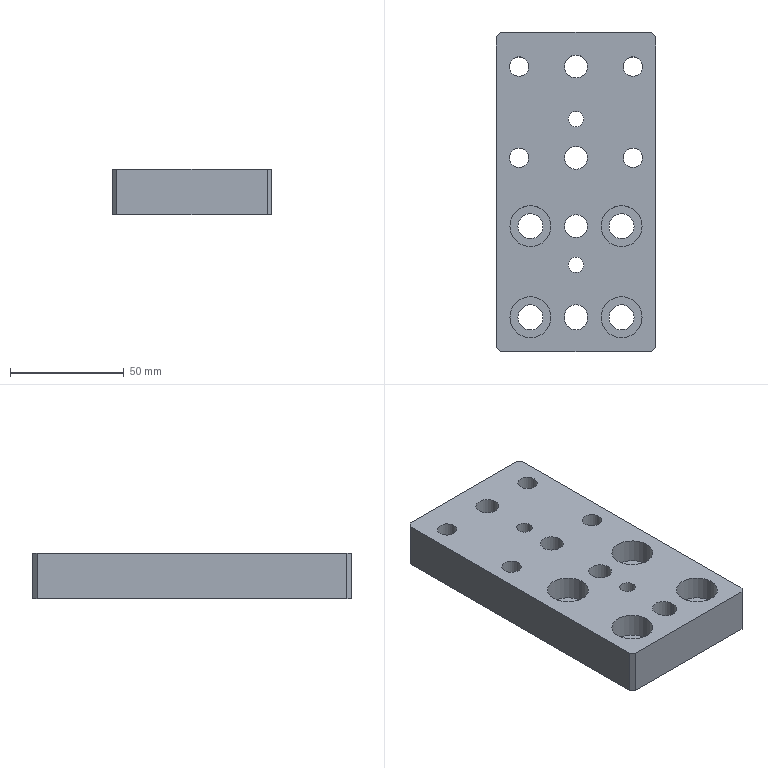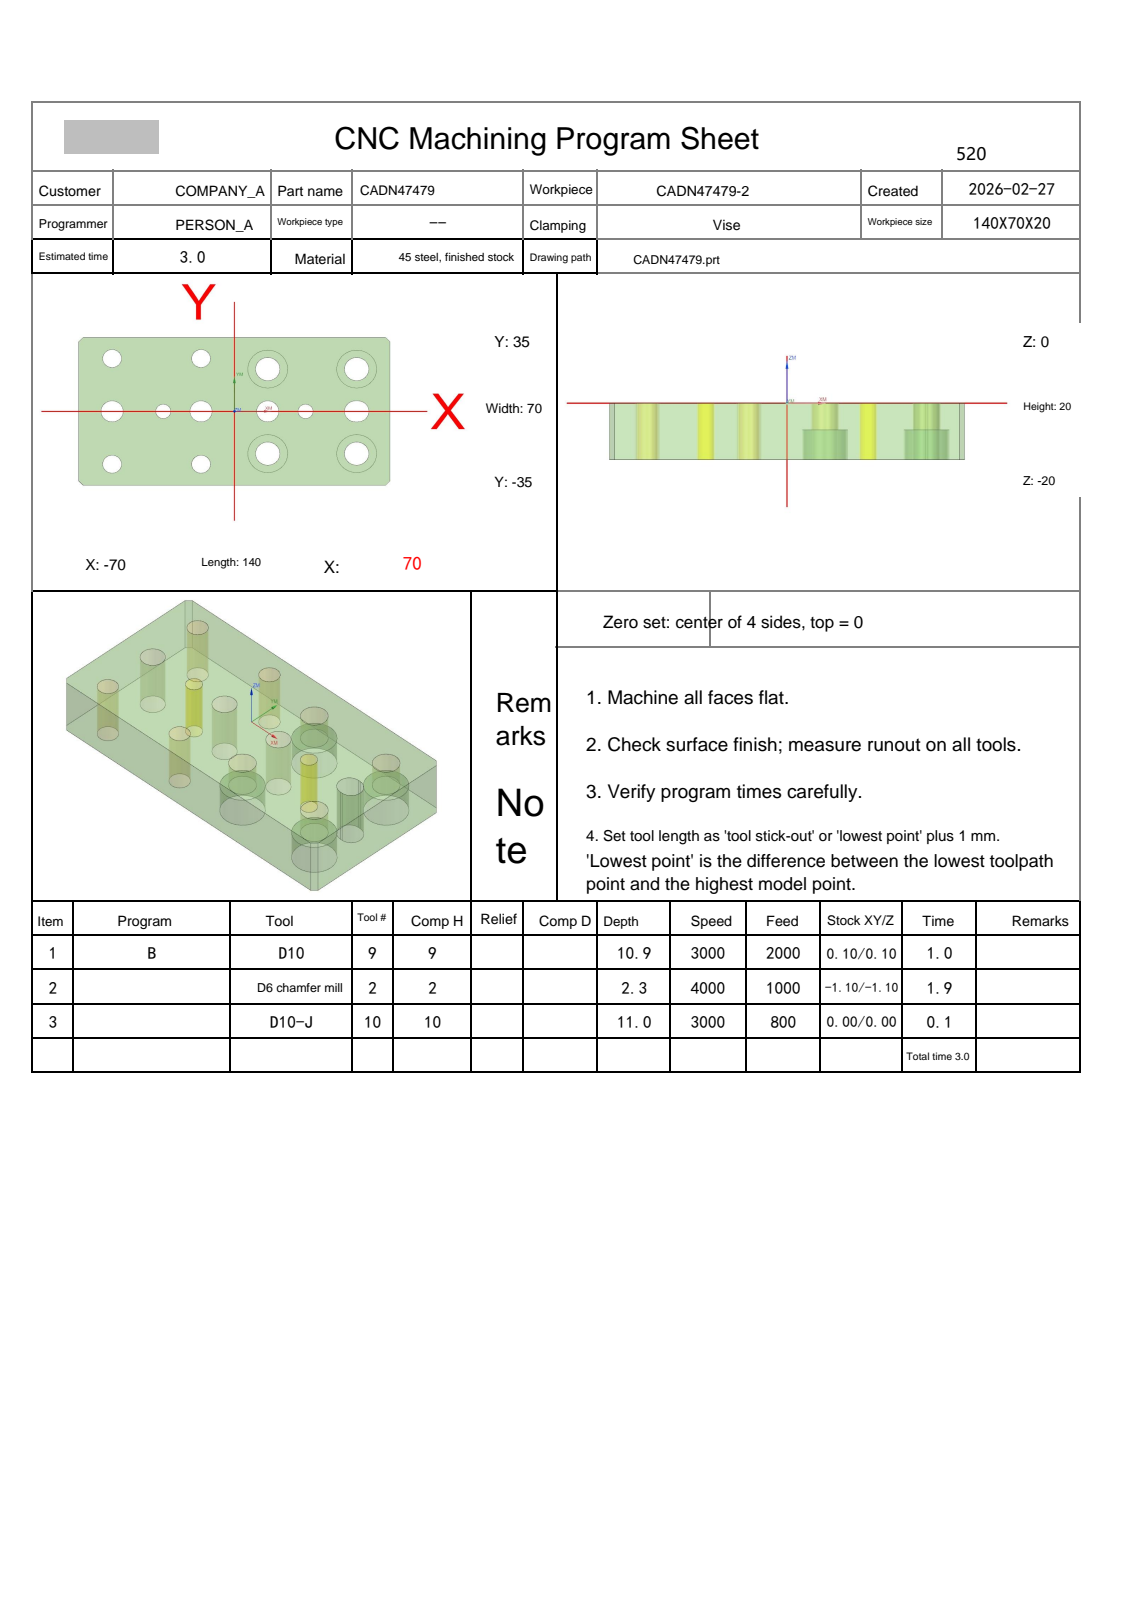NC program | NX | posted by the shop | part box 70 x 140 x 20 mm
Whole program:
%
O0001
(Machine time: 3.57 MIN)
(===Total Tool:3===)
(T9=D10     D=10.  R=0.   D-  H09 Z=-10.9 )
(T2=D6 chamfer mill   D=6.   R=0.   D-  H02 Z=-2.3  )
(T10=D10-J  D=10.  R=0.   D-  H10 Z=-11.  )
G80 G90 G17 G49 G40
G91 G28 Z0
M01
N1 T09 M06
(D10  D=10. R=0. H=09 ce=0.10 di=0.10)
G00 G90 G54 X65.242 Y44.97 M03 S3000
G43 H09 Z30.
M08
Z-.5
G01 X71.606 Y38.606 F2000.
X73.606 Y36.606
X79.97 Y30.242
G00 Z-1.
G01 X73.606 Y36.606
X71.606 Y38.606
X65.242 Y44.97
G00 Z-1.5
G01 X71.606 Y38.606
X73.606 Y36.606
X79.97 Y30.242
G00 Z-2.
G01 X73.606 Y36.606
X71.606 Y38.606
X65.242 Y44.97
G00 Z-2.5
G01 X71.606 Y38.606
X73.606 Y36.606
X79.97 Y30.242
G00 Z-3.
G01 X73.606 Y36.606
X71.606 Y38.606
X65.242 Y44.97
G00 Z-3.5
G01 X71.606 Y38.606
X73.606 Y36.606
X79.97 Y30.242
G00 Z-4.
G01 X73.606 Y36.606
X71.606 Y38.606
X65.242 Y44.97
G00 Z-4.5
G01 X71.606 Y38.606
X73.606 Y36.606
X79.97 Y30.242
G00 Z-5.
G01 X73.606 Y36.606
X71.606 Y38.606
X65.242 Y44.97
G00 Z-5.5
G01 X71.606 Y38.606
X73.606 Y36.606
X79.97 Y30.242
G00 Z-6.
G01 X73.606 Y36.606
X71.606 Y38.606
X65.242 Y44.97
G00 Z-6.5
G01 X71.606 Y38.606
X73.606 Y36.606
X79.97 Y30.242
G00 Z-7.
G01 X73.606 Y36.606
X71.606 Y38.606
X65.242 Y44.97
G00 Z-7.5
G01 X71.606 Y38.606
X73.606 Y36.606
X79.97 Y30.242
G00 Z-8.
G01 X73.606 Y36.606
X71.606 Y38.606
X65.242 Y44.97
G00 Z-8.5
G01 X71.606 Y38.606
X73.606 Y36.606
X79.97 Y30.242
G00 Z-9.
G01 X73.606 Y36.606
X71.606 Y38.606
X65.242 Y44.97
G00 Z-9.5
G01 X71.606 Y38.606
X73.606 Y36.606
X79.97 Y30.242
G00 Z-10.
G01 X73.606 Y36.606
X71.606 Y38.606
X65.242 Y44.97
G00 Z-10.5
G01 X71.606 Y38.606
X73.606 Y36.606
X79.97 Y30.242
G00 Z-10.9
G01 X73.606 Y36.606
X71.606 Y38.606
X65.242 Y44.97
G00 Z30.
X79.97 Y-30.242
Z-.5
G01 X73.606 Y-36.606
X71.606 Y-38.606
X65.242 Y-44.97
G00 Z-1.
G01 X71.606 Y-38.606
X73.606 Y-36.606
X79.97 Y-30.242
G00 Z-1.5
G01 X73.606 Y-36.606
X71.606 Y-38.606
X65.242 Y-44.97
G00 Z-2.
G01 X71.606 Y-38.606
X73.606 Y-36.606
X79.97 Y-30.242
G00 Z-2.5
G01 X73.606 Y-36.606
X71.606 Y-38.606
X65.242 Y-44.97
G00 Z-3.
G01 X71.606 Y-38.606
X73.606 Y-36.606
X79.97 Y-30.242
G00 Z-3.5
G01 X73.606 Y-36.606
X71.606 Y-38.606
X65.242 Y-44.97
G00 Z-4.
G01 X71.606 Y-38.606
X73.606 Y-36.606
X79.97 Y-30.242
G00 Z-4.5
G01 X73.606 Y-36.606
X71.606 Y-38.606
X65.242 Y-44.97
G00 Z-5.
G01 X71.606 Y-38.606
X73.606 Y-36.606
X79.97 Y-30.242
G00 Z-5.5
G01 X73.606 Y-36.606
X71.606 Y-38.606
X65.242 Y-44.97
G00 Z-6.
G01 X71.606 Y-38.606
X73.606 Y-36.606
X79.97 Y-30.242
G00 Z-6.5
G01 X73.606 Y-36.606
X71.606 Y-38.606
X65.242 Y-44.97
G00 Z-7.
G01 X71.606 Y-38.606
X73.606 Y-36.606
X79.97 Y-30.242
G00 Z-7.5
G01 X73.606 Y-36.606
X71.606 Y-38.606
X65.242 Y-44.97
G00 Z-8.
G01 X71.606 Y-38.606
X73.606 Y-36.606
X79.97 Y-30.242
G00 Z-8.5
G01 X73.606 Y-36.606
X71.606 Y-38.606
X65.242 Y-44.97
G00 Z-9.
G01 X71.606 Y-38.606
X73.606 Y-36.606
X79.97 Y-30.242
G00 Z-9.5
G01 X73.606 Y-36.606
X71.606 Y-38.606
X65.242 Y-44.97
G00 Z-10.
G01 X71.606 Y-38.606
X73.606 Y-36.606
X79.97 Y-30.242
G00 Z-10.5
G01 X73.606 Y-36.606
X71.606 Y-38.606
X65.242 Y-44.97
G00 Z-10.9
G01 X71.606 Y-38.606
X73.606 Y-36.606
X79.97 Y-30.242
G00 Z30.
X-65.242 Y-44.97
Z-.5
G01 X-71.606 Y-38.606
X-73.606 Y-36.606
X-79.97 Y-30.242
G00 Z-1.
G01 X-73.606 Y-36.606
X-71.606 Y-38.606
X-65.242 Y-44.97
G00 Z-1.5
G01 X-71.606 Y-38.606
X-73.606 Y-36.606
X-79.97 Y-30.242
G00 Z-2.
G01 X-73.606 Y-36.606
X-71.606 Y-38.606
X-65.242 Y-44.97
G00 Z-2.5
G01 X-71.606 Y-38.606
X-73.606 Y-36.606
X-79.97 Y-30.242
G00 Z-3.
G01 X-73.606 Y-36.606
X-71.606 Y-38.606
X-65.242 Y-44.97
G00 Z-3.5
G01 X-71.606 Y-38.606
X-73.606 Y-36.606
X-79.97 Y-30.242
G00 Z-4.
G01 X-73.606 Y-36.606
X-71.606 Y-38.606
X-65.242 Y-44.97
G00 Z-4.5
G01 X-71.606 Y-38.606
X-73.606 Y-36.606
X-79.97 Y-30.242
G00 Z-5.
G01 X-73.606 Y-36.606
X-71.606 Y-38.606
X-65.242 Y-44.97
G00 Z-5.5
G01 X-71.606 Y-38.606
X-73.606 Y-36.606
X-79.97 Y-30.242
G00 Z-6.
G01 X-73.606 Y-36.606
X-71.606 Y-38.606
X-65.242 Y-44.97
G00 Z-6.5
G01 X-71.606 Y-38.606
X-73.606 Y-36.606
X-79.97 Y-30.242
G00 Z-7.
G01 X-73.606 Y-36.606
X-71.606 Y-38.606
X-65.242 Y-44.97
G00 Z-7.5
G01 X-71.606 Y-38.606
X-73.606 Y-36.606
X-79.97 Y-30.242
G00 Z-8.
G01 X-73.606 Y-36.606
X-71.606 Y-38.606
X-65.242 Y-44.97
G00 Z-8.5
G01 X-71.606 Y-38.606
X-73.606 Y-36.606
X-79.97 Y-30.242
G00 Z-9.
G01 X-73.606 Y-36.606
X-71.606 Y-38.606
X-65.242 Y-44.97
G00 Z-9.5
G01 X-71.606 Y-38.606
X-73.606 Y-36.606
X-79.97 Y-30.242
G00 Z-10.
G01 X-73.606 Y-36.606
X-71.606 Y-38.606
X-65.242 Y-44.97
G00 Z-10.5
G01 X-71.606 Y-38.606
X-73.606 Y-36.606
X-79.97 Y-30.242
G00 Z-10.9
G01 X-73.606 Y-36.606
X-71.606 Y-38.606
X-65.242 Y-44.97
G00 Z30.
X-79.97 Y30.242
Z-.5
G01 X-73.606 Y36.606
X-71.606 Y38.606
X-65.242 Y44.97
G00 Z-1.
G01 X-71.606 Y38.606
X-73.606 Y36.606
X-79.97 Y30.242
G00 Z-1.5
G01 X-73.606 Y36.606
X-71.606 Y38.606
X-65.242 Y44.97
G00 Z-2.
G01 X-71.606 Y38.606
X-73.606 Y36.606
X-79.97 Y30.242
G00 Z-2.5
G01 X-73.606 Y36.606
X-71.606 Y38.606
X-65.242 Y44.97
G00 Z-3.
G01 X-71.606 Y38.606
X-73.606 Y36.606
X-79.97 Y30.242
G00 Z-3.5
G01 X-73.606 Y36.606
X-71.606 Y38.606
X-65.242 Y44.97
G00 Z-4.
G01 X-71.606 Y38.606
X-73.606 Y36.606
X-79.97 Y30.242
G00 Z-4.5
G01 X-73.606 Y36.606
X-71.606 Y38.606
X-65.242 Y44.97
G00 Z-5.
G01 X-71.606 Y38.606
X-73.606 Y36.606
X-79.97 Y30.242
G00 Z-5.5
G01 X-73.606 Y36.606
X-71.606 Y38.606
X-65.242 Y44.97
G00 Z-6.
G01 X-71.606 Y38.606
X-73.606 Y36.606
X-79.97 Y30.242
G00 Z-6.5
G01 X-73.606 Y36.606
X-71.606 Y38.606
X-65.242 Y44.97
G00 Z-7.
G01 X-71.606 Y38.606
X-73.606 Y36.606
X-79.97 Y30.242
G00 Z-7.5
G01 X-73.606 Y36.606
X-71.606 Y38.606
X-65.242 Y44.97
G00 Z-8.
G01 X-71.606 Y38.606
X-73.606 Y36.606
X-79.97 Y30.242
G00 Z-8.5
G01 X-73.606 Y36.606
X-71.606 Y38.606
X-65.242 Y44.97
G00 Z-9.
G01 X-71.606 Y38.606
X-73.606 Y36.606
X-79.97 Y30.242
G00 Z-9.5
G01 X-73.606 Y36.606
X-71.606 Y38.606
X-65.242 Y44.97
G00 Z-10.
G01 X-71.606 Y38.606
X-73.606 Y36.606
X-79.97 Y30.242
G00 Z-10.5
G01 X-73.606 Y36.606
X-71.606 Y38.606
X-65.242 Y44.97
G00 Z-10.9
G01 X-71.606 Y38.606
X-73.606 Y36.606
X-79.97 Y30.242
G00 Z30.
G91 G28 Z0.0
M05
M09
G91 G28 Z0.0
M01
N2 T02 M06
(D6 chamfer mill  D=6. R=0. H=02 ce=-1.00 di=-0.80)
G00 G90 G54 X33.5 Y.995 M03 S4000
G43 H02 Z30.
M08
Z-1.1
G01 Z-1.6 F300.
Y1.3
G03 X32. Y2.8 I-1.5 J0.0
X29.2 Y0.0 I0.0 J-2.8
X32. Y-2.8 I2.8 J0.0
X34.8 Y0.0 I0.0 J2.8
X32. Y2.8 I-2.8 J0.0
X30.5 Y1.3 I0.0 J-1.5
G01 Y.995
Z-1.1
G00 Z30.
X-30.5
Z-1.1
G01 Z-1.6
Y1.3
G03 X-32. Y2.8 I-1.5 J0.0
X-34.8 Y0.0 I0.0 J-2.8
X-32. Y-2.8 I2.8 J0.0
X-29.2 Y0.0 I0.0 J2.8
X-32. Y2.8 I-2.8 J0.0
X-33.5 Y1.3 I0.0 J-1.5
G01 Y.995
Z-1.1
G00 Z30.
G00 G90 X-52.258 Y-24.223 M03 S3000
Z30.
Z-1.
G01 Z-1.5 F400.
X-52. Y-24.15
G03 X-55. Y-21.15 I-3. J0.0
X-58.85 Y-25. I0.0 J-3.85
X-55. Y-28.85 I3.85 J0.0
X-51.15 Y-25. I0.0 J3.85
X-55. Y-21.15 I-3.85 J0.0
X-58. Y-24.15 I0.0 J-3.
G01 X-57.742 Y-24.223
Z-1.
G00 Z30.
X-12.258
Z-1.
G01 Z-1.5
X-12. Y-24.15
G03 X-15. Y-21.15 I-3. J0.0
X-18.85 Y-25. I0.0 J-3.85
X-15. Y-28.85 I3.85 J0.0
X-11.15 Y-25. I0.0 J3.85
X-15. Y-21.15 I-3.85 J0.0
X-18. Y-24.15 I0.0 J-3.
G01 X-17.742 Y-24.223
Z-1.
G00 Z30.
X-12.258 Y25.777
Z-1.
G01 Z-1.5
X-12. Y25.85
G03 X-15. Y28.85 I-3. J0.0
X-18.85 Y25. I0.0 J-3.85
X-15. Y21.15 I3.85 J0.0
X-11.15 Y25. I0.0 J3.85
X-15. Y28.85 I-3.85 J0.0
X-18. Y25.85 I0.0 J-3.
G01 X-17.742 Y25.777
Z-1.
G00 Z30.
X-52.258
Z-1.
G01 Z-1.5
X-52. Y25.85
G03 X-55. Y28.85 I-3. J0.0
X-58.85 Y25. I0.0 J-3.85
X-55. Y21.15 I3.85 J0.0
X-51.15 Y25. I0.0 J3.85
X-55. Y28.85 I-3.85 J0.0
X-58. Y25.85 I0.0 J-3.
G01 X-57.742 Y25.777
Z-1.
G00 Z30.
G00 G90 X18. Y1.3 M03 S3000
Z30.
Z-.5
G01 Z-1. F600.
G03 X15. Y4.3 I-3. J0.0
X10.7 Y0.0 I0.0 J-4.3
X15. Y-4.3 I4.3 J0.0
X19.3 Y0.0 I0.0 J4.3
X15. Y4.3 I-4.3 J0.0
X12. Y1.3 I0.0 J-3.
G01 Z-.5
G00 Z30.
X-12.
Z-.5
G01 Z-1.
G03 X-15. Y4.3 I-3. J0.0
X-19.3 Y0.0 I0.0 J-4.3
X-15. Y-4.3 I4.3 J0.0
X-10.7 Y0.0 I0.0 J4.3
X-15. Y4.3 I-4.3 J0.0
X-18. Y1.3 I0.0 J-3.
G01 Z-.5
G00 Z30.
X-52.
Z-.5
G01 Z-1.
G03 X-55. Y4.3 I-3. J0.0
X-59.3 Y0.0 I0.0 J-4.3
X-55. Y-4.3 I4.3 J0.0
X-50.7 Y0.0 I0.0 J4.3
X-55. Y4.3 I-4.3 J0.0
X-58. Y1.3 I0.0 J-3.
G01 Z-.5
G00 Z30.
G00 G90 X17.466 Y-19.589 M03 S3000
Z30.
Z-1.8
G01 Z-2.3 F600.
X18. Y-19.5
G03 X15. Y-16.5 I-3. J0.0
X11.5 Y-20. I0.0 J-3.5
X15. Y-23.5 I3.5 J0.0
X18.5 Y-20. I0.0 J3.5
X15. Y-16.5 I-3.5 J0.0
X12. Y-19.5 I0.0 J-3.
G01 X12.534 Y-19.589
Z-1.8
G00 Z30.
X57.466
Z-1.8
G01 Z-2.3
X58. Y-19.5
G03 X55. Y-16.5 I-3. J0.0
X51.5 Y-20. I0.0 J-3.5
X55. Y-23.5 I3.5 J0.0
X58.5 Y-20. I0.0 J3.5
X55. Y-16.5 I-3.5 J0.0
X52. Y-19.5 I0.0 J-3.
G01 X52.534 Y-19.589
Z-1.8
G00 Z30.
X57.466 Y20.411
Z-1.8
G01 Z-2.3
X58. Y20.5
G03 X55. Y23.5 I-3. J0.0
X51.5 Y20. I0.0 J-3.5
X55. Y16.5 I3.5 J0.0
X58.5 Y20. I0.0 J3.5
X55. Y23.5 I-3.5 J0.0
X52. Y20.5 I0.0 J-3.
G01 X52.534 Y20.411
Z-1.8
G00 Z30.
X17.466
Z-1.8
G01 Z-2.3
X18. Y20.5
G03 X15. Y23.5 I-3. J0.0
X11.5 Y20. I0.0 J-3.5
X15. Y16.5 I3.5 J0.0
X18.5 Y20. I0.0 J3.5
X15. Y23.5 I-3.5 J0.0
X12. Y20.5 I0.0 J-3.
G01 X12.534 Y20.411
Z-1.8
G00 Z30.
G00 G90 X-.386 Y36.227 M03 S3500
Z30.
Z.172
G01 Z-1.2 F1000.
G03 X-.1 Y36.027 I1.286 J1.532
G01 X-.054 Y35.997
X0.0 Y36.
X68.
X68.259 Y35.966
X68.5 Y35.866
X68.707 Y35.707
X70.707 Y33.707
X70.866 Y33.5
X70.966 Y33.259
X71. Y33.
Y-33.
X70.966 Y-33.259
X70.866 Y-33.5
X70.707 Y-33.707
X68.707 Y-35.707
X68.5 Y-35.866
X68.259 Y-35.966
X68. Y-36.
X-68.
X-68.259 Y-35.966
X-68.5 Y-35.866
X-68.707 Y-35.707
X-70.707 Y-33.707
X-70.866 Y-33.5
X-70.966 Y-33.259
X-71. Y-33.
Y33.
X-70.966 Y33.259
X-70.866 Y33.5
X-70.707 Y33.707
X-68.707 Y35.707
X-68.5 Y35.866
X-68.259 Y35.966
X-68. Y36.
X0.0
X.054 Y35.997
X.1 Y36.027
G03 X.386 Y36.227 I-1. J1.732
G01 Z.172
G00 Z10.
X-54.599 Y28.053
Z.232
G01 Z-1.2
G03 X-54.898 Y28.231 I-1.167 J-1.624
G01 X-54.946 Y28.257
X-55. Y28.25
G03 X-58.25 Y25. I0.0 J-3.25
X-55. Y21.75 I3.25 J0.0
X-51.75 Y25. I0.0 J3.25
X-55. Y28.25 I-3.25 J0.0
G01 X-55.054 Y28.257
X-55.102 Y28.231
G03 X-55.401 Y28.053 I.868 J-1.802
G01 Z.232
G00 Z10.
X-54.6 Y3.799
Z.225
G01 Z-1.2
G03 X-54.898 Y3.98 I-1.183 J-1.613
G01 X-54.946 Y4.006
X-55. Y4.
G03 X-59. Y0.0 I0.0 J-4.
X-55. Y-4. I4. J0.0
X-51. Y0.0 I0.0 J4.
X-55. Y4. I-4. J0.0
G01 X-55.054 Y4.006
X-55.102 Y3.98
G03 X-55.4 Y3.799 I.885 J-1.794
G01 Z.225
G00 Z10.
X-54.599 Y-21.947
Z.232
G01 Z-1.2
G03 X-54.898 Y-21.769 I-1.167 J-1.624
G01 X-54.946 Y-21.743
X-55. Y-21.75
G03 X-58.25 Y-25. I0.0 J-3.25
X-55. Y-28.25 I3.25 J0.0
X-51.75 Y-25. I0.0 J3.25
X-55. Y-21.75 I-3.25 J0.0
G01 X-55.054 Y-21.743
X-55.102 Y-21.769
G03 X-55.401 Y-21.947 I.868 J-1.802
G01 Z.232
G00 Z10.
X-14.599
Z.232
G01 Z-1.2
G03 X-14.898 Y-21.769 I-1.167 J-1.624
G01 X-14.946 Y-21.743
X-15. Y-21.75
G03 X-18.25 Y-25. I0.0 J-3.25
X-15. Y-28.25 I3.25 J0.0
X-11.75 Y-25. I0.0 J3.25
X-15. Y-21.75 I-3.25 J0.0
G01 X-15.054 Y-21.743
X-15.102 Y-21.769
G03 X-15.401 Y-21.947 I.868 J-1.802
G01 Z.232
G00 Z10.
X-14.6 Y3.799
Z.225
G01 Z-1.2
G03 X-14.898 Y3.98 I-1.183 J-1.613
G01 X-14.946 Y4.006
X-15. Y4.
G03 X-19. Y0.0 I0.0 J-4.
X-15. Y-4. I4. J0.0
X-11. Y0.0 I0.0 J4.
X-15. Y4. I-4. J0.0
G01 X-15.054 Y4.006
X-15.102 Y3.98
G03 X-15.4 Y3.799 I.885 J-1.794
G01 Z.225
G00 Z10.
X-31.596 Y2.208
Z.252
G01 Z-1.2
G03 X-31.898 Y2.382 I-1.147 J-1.638
G01 X-31.946 Y2.408
X-32. Y2.4
G03 X-34.4 Y0.0 I0.0 J-2.4
X-32. Y-2.4 I2.4 J0.0
X-29.6 Y0.0 I0.0 J2.4
X-32. Y2.4 I-2.4 J0.0
G01 X-32.054 Y2.408
X-32.102 Y2.382
G03 X-32.404 Y2.208 I.845 J-1.813
G01 Z.252
G00 Z10.
X-14.599 Y28.053
Z.232
G01 Z-1.2
G03 X-14.898 Y28.231 I-1.167 J-1.624
G01 X-14.946 Y28.257
X-15. Y28.25
G03 X-18.25 Y25. I0.0 J-3.25
X-15. Y21.75 I3.25 J0.0
X-11.75 Y25. I0.0 J3.25
X-15. Y28.25 I-3.25 J0.0
G01 X-15.054 Y28.257
X-15.102 Y28.231
G03 X-15.401 Y28.053 I.868 J-1.802
G01 Z.232
G00 Z10.
X15.4 Y24.299
Z.224
G01 Z-1.2
G03 X15.102 Y24.48 I-1.183 J-1.613
G01 X15.054 Y24.506
X15. Y24.5
G03 X10.5 Y20. I0.0 J-4.5
X15. Y15.5 I4.5 J0.0
X19.5 Y20. I0.0 J4.5
X15. Y24.5 I-4.5 J0.0
G01 X14.946 Y24.506
X14.898 Y24.48
G03 X14.6 Y24.299 I.885 J-1.794
G01 Z.224
G00 Z10.
X15.4 Y3.799
Z.225
G01 Z-1.2
G03 X15.102 Y3.98 I-1.183 J-1.613
G01 X15.054 Y4.006
X15. Y4.
G03 X11. Y0.0 I0.0 J-4.
X15. Y-4. I4. J0.0
X19. Y0.0 I0.0 J4.
X15. Y4. I-4. J0.0
G01 X14.946 Y4.006
X14.898 Y3.98
G03 X14.6 Y3.799 I.885 J-1.794
G01 Z.225
G00 Z10.
X15.4 Y-15.701
Z.224
G01 Z-1.2
G03 X15.102 Y-15.52 I-1.183 J-1.613
G01 X15.054 Y-15.494
X15. Y-15.5
G03 X10.5 Y-20. I0.0 J-4.5
X15. Y-24.5 I4.5 J0.0
X19.5 Y-20. I0.0 J4.5
X15. Y-15.5 I-4.5 J0.0
G01 X14.946 Y-15.494
X14.898 Y-15.52
G03 X14.6 Y-15.701 I.885 J-1.794
G01 Z.224
G00 Z10.
X32.404 Y2.208
Z.252
G01 Z-1.2
G03 X32.102 Y2.382 I-1.147 J-1.638
G01 X32.054 Y2.408
X32. Y2.4
G03 X29.6 Y0.0 I0.0 J-2.4
X32. Y-2.4 I2.4 J0.0
X34.4 Y0.0 I0.0 J2.4
X32. Y2.4 I-2.4 J0.0
G01 X31.946 Y2.408
X31.898 Y2.382
G03 X31.596 Y2.208 I.845 J-1.813
G01 Z.252
G00 Z10.
X55.4 Y24.299
Z.224
G01 Z-1.2
G03 X55.102 Y24.48 I-1.183 J-1.613
G01 X55.054 Y24.506
X55. Y24.5
G03 X50.5 Y20. I0.0 J-4.5
X55. Y15.5 I4.5 J0.0
X59.5 Y20. I0.0 J4.5
X55. Y24.5 I-4.5 J0.0
G01 X54.946 Y24.506
X54.898 Y24.48
G03 X54.6 Y24.299 I.885 J-1.794
G01 Z.224
G00 Z10.
X54.614 Y-3.773
Z.172
G01 Z-1.2
G03 X54.9 Y-3.973 I1.286 J1.532
G01 X54.946 Y-4.003
X55. Y-4.
X55.5
G03 X59.5 Y0.0 I0.0 J4.
X55.5 Y4. I-4. J0.0
G01 X54.5
G03 X50.5 Y0.0 I0.0 J-4.
X54.5 Y-4. I4. J0.0
G01 X55.
X55.054 Y-4.003
X55.1 Y-3.973
G03 X55.386 Y-3.773 I-1. J1.732
G01 Z.172
G00 Z2.55
X55.4 Y-15.701
Z.224
G01 Z-1.2
G03 X55.102 Y-15.52 I-1.183 J-1.613
G01 X55.054 Y-15.494
X55. Y-15.5
G03 X50.5 Y-20. I0.0 J-4.5
X55. Y-24.5 I4.5 J0.0
X59.5 Y-20. I0.0 J4.5
X55. Y-15.5 I-4.5 J0.0
G01 X54.946 Y-15.494
X54.898 Y-15.52
G03 X54.6 Y-15.701 I.885 J-1.794
G01 Z.224
G00 Z30.
G91 G28 Z0.0
M05
M09
G91 G28 Z0.0
M01
N3 T10 M06
(D10-J  D=10. R=0. H=10 ce=0.00 di=0.00)
G00 G90 G54 X67.293 Y42.778 M03 S3000
G43 H10 Z30.
M08
Z-10.
G01 Z-11. F800.
X71.536 Y38.536
X73.536 Y36.536
X77.778 Y32.293
Z-10.
G00 Z30.
Y-32.293
Z-10.
G01 Z-11.
X73.536 Y-36.536
X71.536 Y-38.536
X67.293 Y-42.778
Z-10.
G00 Z30.
X-67.293
Z-10.
G01 Z-11.
X-71.536 Y-38.536
X-73.536 Y-36.536
X-77.778 Y-32.293
Z-10.
G00 Z30.
Y32.293
Z-10.
G01 Z-11.
X-73.536 Y36.536
X-71.536 Y38.536
X-67.293 Y42.778
Z-10.
G00 Z30.
M05
M09
G91 G28 Z0.0
G91 G28 Y0.0
M30
%